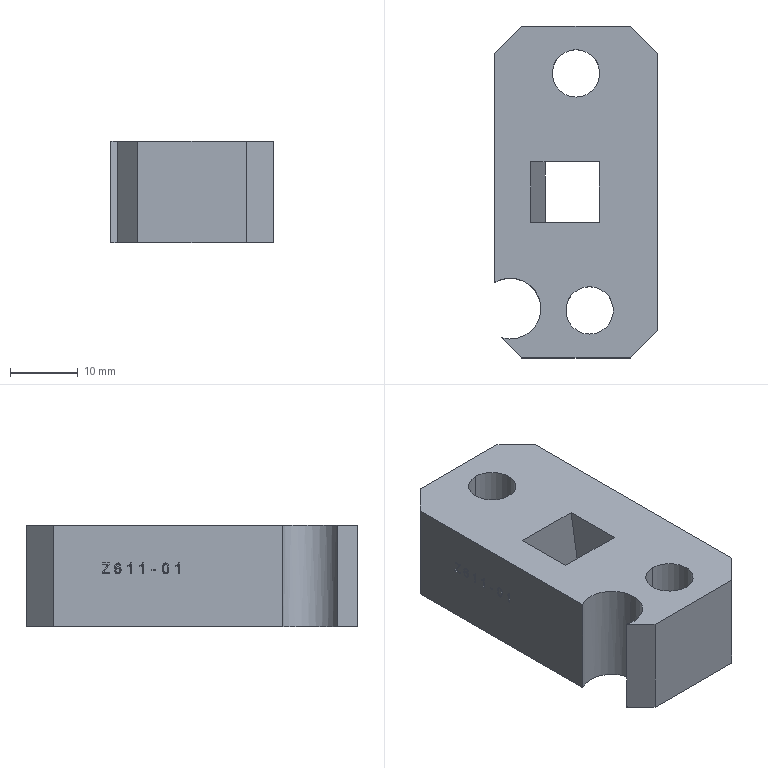Part | Creo | 1 solid | 125 faces | box 24 x 49 x 15 mm | volume 13080 mm3 | other 63 | plane 52 | cylinder 10 | commonest cylinder face diameters 7 x4 11 x4 9 x1 21.664 x1